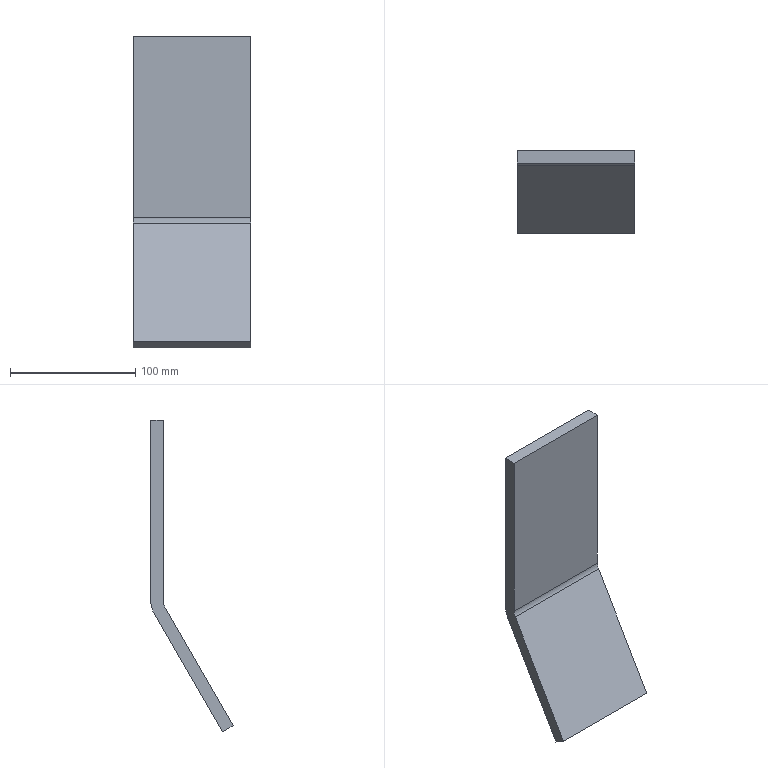Part | STEP file | VD-SYL0380DJ1006_1_4-5_VD-SYL03 | 1 solid | 10 faces | box 94 x 65.818 x 249 mm | volume 245764 mm3 | plane 8 | cylinder 2 | commonest cylinder face diameters 20 x1 40 x1
STEP:
#1=CARTESIAN_POINT('',(-47.,0.,-144.641));
#2=VERTEX_POINT('',#1);
#3=CARTESIAN_POINT('',(47.,0.,-144.641));
#4=VERTEX_POINT('',#3);
#5=CARTESIAN_POINT('',(-47.,0.,-144.641));
#6=DIRECTION('',(1.,0.,0.));
#7=VECTOR('',#6,1000.);
#8=LINE('',#5,#7);
#9=EDGE_CURVE('',#2,#4,#8,.T.);
#10=ORIENTED_EDGE('',*,*,#9,.F.);
#11=CARTESIAN_POINT('',(-47.,0.,0.));
#12=VERTEX_POINT('',#11);
#13=CARTESIAN_POINT('',(-47.,0.,0.));
#14=DIRECTION('',(0.,0.,-1.));
#15=VECTOR('',#14,1000.);
#16=LINE('',#13,#15);
#17=EDGE_CURVE('',#12,#2,#16,.T.);
#18=ORIENTED_EDGE('',*,*,#17,.F.);
#19=CARTESIAN_POINT('',(47.,0.,0.));
#20=VERTEX_POINT('',#19);
#21=CARTESIAN_POINT('',(47.,0.,0.));
#22=DIRECTION('',(-1.,0.,0.));
#23=VECTOR('',#22,1000.);
#24=LINE('',#21,#23);
#25=EDGE_CURVE('',#20,#12,#24,.T.);
#26=ORIENTED_EDGE('',*,*,#25,.F.);
#27=CARTESIAN_POINT('',(47.,0.,-144.641));
#28=DIRECTION('',(0.,0.,1.));
#29=VECTOR('',#28,1000.);
#30=LINE('',#27,#29);
#31=EDGE_CURVE('',#4,#20,#30,.T.);
#32=ORIENTED_EDGE('',*,*,#31,.F.);
#33=EDGE_LOOP('',(#10,#18,#26,#32));
#34=FACE_OUTER_BOUND('',#33,.T.);
#35=CARTESIAN_POINT('',(-47.,0.,-150.));
#36=DIRECTION('',(0.,1.,0.));
#37=DIRECTION('',(1.,0.,0.));
#38=AXIS2_PLACEMENT_3D('',#35,#36,#37);
#39=PLANE('',#38);
#40=ADVANCED_FACE('',(#34),#39,.T.);
#41=CARTESIAN_POINT('',(-47.,-2.679,-154.641));
#42=VERTEX_POINT('',#41);
#43=CARTESIAN_POINT('',(-47.,-20.,-144.641));
#44=DIRECTION('',(-1.,0.,0.));
#45=DIRECTION('',(0.,1.,0.));
#46=AXIS2_PLACEMENT_3D('',#43,#44,#45);
#47=CIRCLE('',#46,20.);
#48=EDGE_CURVE('',#2,#42,#47,.T.);
#49=ORIENTED_EDGE('',*,*,#48,.T.);
#50=CARTESIAN_POINT('',(-47.,-57.158,-249.));
#51=VERTEX_POINT('',#50);
#52=CARTESIAN_POINT('',(-47.,-2.679,-154.641));
#53=DIRECTION('',(0.,-0.5,-0.866));
#54=VECTOR('',#53,1000.);
#55=LINE('',#52,#54);
#56=EDGE_CURVE('',#42,#51,#55,.T.);
#57=ORIENTED_EDGE('',*,*,#56,.T.);
#58=CARTESIAN_POINT('',(-47.,-65.818,-244.));
#59=VERTEX_POINT('',#58);
#60=CARTESIAN_POINT('',(-47.,-57.158,-249.));
#61=DIRECTION('',(0.,-0.866,0.5));
#62=VECTOR('',#61,1000.);
#63=LINE('',#60,#62);
#64=EDGE_CURVE('',#51,#59,#63,.T.);
#65=ORIENTED_EDGE('',*,*,#64,.T.);
#66=CARTESIAN_POINT('',(-47.,-11.34,-149.641));
#67=VERTEX_POINT('',#66);
#68=CARTESIAN_POINT('',(-47.,-65.818,-244.));
#69=DIRECTION('',(0.,0.5,0.866));
#70=VECTOR('',#69,1000.);
#71=LINE('',#68,#70);
#72=EDGE_CURVE('',#59,#67,#71,.T.);
#73=ORIENTED_EDGE('',*,*,#72,.T.);
#74=CARTESIAN_POINT('',(-47.,-10.,-144.641));
#75=VERTEX_POINT('',#74);
#76=CARTESIAN_POINT('',(-47.,-20.,-144.641));
#77=DIRECTION('',(1.,0.,0.));
#78=DIRECTION('',(0.,0.866,-0.5));
#79=AXIS2_PLACEMENT_3D('',#76,#77,#78);
#80=CIRCLE('',#79,10.);
#81=EDGE_CURVE('',#67,#75,#80,.T.);
#82=ORIENTED_EDGE('',*,*,#81,.T.);
#83=CARTESIAN_POINT('',(-47.,-10.,0.));
#84=VERTEX_POINT('',#83);
#85=CARTESIAN_POINT('',(-47.,-10.,0.));
#86=DIRECTION('',(0.,0.,-1.));
#87=VECTOR('',#86,1000.);
#88=LINE('',#85,#87);
#89=EDGE_CURVE('',#84,#75,#88,.T.);
#90=ORIENTED_EDGE('',*,*,#89,.F.);
#91=CARTESIAN_POINT('',(-47.,-10.,0.));
#92=DIRECTION('',(0.,1.,0.));
#93=VECTOR('',#92,1000.);
#94=LINE('',#91,#93);
#95=EDGE_CURVE('',#84,#12,#94,.T.);
#96=ORIENTED_EDGE('',*,*,#95,.T.);
#97=ORIENTED_EDGE('',*,*,#17,.T.);
#98=EDGE_LOOP('',(#49,#57,#65,#73,#82,#90,#96,#97));
#99=FACE_OUTER_BOUND('',#98,.T.);
#100=CARTESIAN_POINT('',(-47.,-5.,-74.33));
#101=DIRECTION('',(-1.,0.,0.));
#102=DIRECTION('',(0.,0.,1.));
#103=AXIS2_PLACEMENT_3D('',#100,#101,#102);
#104=PLANE('',#103);
#105=ADVANCED_FACE('',(#99),#104,.T.);
#106=CARTESIAN_POINT('',(47.,-2.679,-154.641));
#107=VERTEX_POINT('',#106);
#108=CARTESIAN_POINT('',(47.,-2.679,-154.641));
#109=DIRECTION('',(-1.,0.,0.));
#110=VECTOR('',#109,1000.);
#111=LINE('',#108,#110);
#112=EDGE_CURVE('',#107,#42,#111,.T.);
#113=ORIENTED_EDGE('',*,*,#112,.F.);
#114=CARTESIAN_POINT('',(47.,-57.158,-249.));
#115=VERTEX_POINT('',#114);
#116=CARTESIAN_POINT('',(47.,-57.158,-249.));
#117=DIRECTION('',(0.,0.5,0.866));
#118=VECTOR('',#117,1000.);
#119=LINE('',#116,#118);
#120=EDGE_CURVE('',#115,#107,#119,.T.);
#121=ORIENTED_EDGE('',*,*,#120,.F.);
#122=CARTESIAN_POINT('',(-47.,-57.158,-249.));
#123=DIRECTION('',(1.,0.,0.));
#124=VECTOR('',#123,1000.);
#125=LINE('',#122,#124);
#126=EDGE_CURVE('',#51,#115,#125,.T.);
#127=ORIENTED_EDGE('',*,*,#126,.F.);
#128=ORIENTED_EDGE('',*,*,#56,.F.);
#129=EDGE_LOOP('',(#113,#121,#127,#128));
#130=FACE_OUTER_BOUND('',#129,.T.);
#131=CARTESIAN_POINT('',(-47.,-57.158,-249.));
#132=DIRECTION('',(0.,0.866,-0.5));
#133=DIRECTION('',(-1.,0.,0.));
#134=AXIS2_PLACEMENT_3D('',#131,#132,#133);
#135=PLANE('',#134);
#136=ADVANCED_FACE('',(#130),#135,.T.);
#137=ORIENTED_EDGE('',*,*,#64,.F.);
#138=ORIENTED_EDGE('',*,*,#126,.T.);
#139=CARTESIAN_POINT('',(47.,-65.818,-244.));
#140=VERTEX_POINT('',#139);
#141=CARTESIAN_POINT('',(47.,-65.818,-244.));
#142=DIRECTION('',(0.,0.866,-0.5));
#143=VECTOR('',#142,1000.);
#144=LINE('',#141,#143);
#145=EDGE_CURVE('',#140,#115,#144,.T.);
#146=ORIENTED_EDGE('',*,*,#145,.F.);
#147=CARTESIAN_POINT('',(47.,-65.818,-244.));
#148=DIRECTION('',(-1.,0.,0.));
#149=VECTOR('',#148,1000.);
#150=LINE('',#147,#149);
#151=EDGE_CURVE('',#140,#59,#150,.T.);
#152=ORIENTED_EDGE('',*,*,#151,.T.);
#153=EDGE_LOOP('',(#137,#138,#146,#152));
#154=FACE_OUTER_BOUND('',#153,.T.);
#155=CARTESIAN_POINT('',(0.,-61.488,-246.5));
#156=DIRECTION('',(0.,0.5,0.866));
#157=DIRECTION('',(1.,0.,0.));
#158=AXIS2_PLACEMENT_3D('',#155,#156,#157);
#159=PLANE('',#158);
#160=ADVANCED_FACE('',(#154),#159,.F.);
#161=CARTESIAN_POINT('',(47.,-11.34,-149.641));
#162=VERTEX_POINT('',#161);
#163=CARTESIAN_POINT('',(47.,-11.34,-149.641));
#164=DIRECTION('',(0.,-0.5,-0.866));
#165=VECTOR('',#164,1000.);
#166=LINE('',#163,#165);
#167=EDGE_CURVE('',#162,#140,#166,.T.);
#168=ORIENTED_EDGE('',*,*,#167,.F.);
#169=CARTESIAN_POINT('',(-47.,-11.34,-149.641));
#170=DIRECTION('',(1.,0.,0.));
#171=VECTOR('',#170,1000.);
#172=LINE('',#169,#171);
#173=EDGE_CURVE('',#67,#162,#172,.T.);
#174=ORIENTED_EDGE('',*,*,#173,.F.);
#175=ORIENTED_EDGE('',*,*,#72,.F.);
#176=ORIENTED_EDGE('',*,*,#151,.F.);
#177=EDGE_LOOP('',(#168,#174,#175,#176));
#178=FACE_OUTER_BOUND('',#177,.T.);
#179=CARTESIAN_POINT('',(-47.,-65.818,-244.));
#180=DIRECTION('',(0.,0.866,-0.5));
#181=DIRECTION('',(-1.,0.,0.));
#182=AXIS2_PLACEMENT_3D('',#179,#180,#181);
#183=PLANE('',#182);
#184=ADVANCED_FACE('',(#178),#183,.F.);
#185=ORIENTED_EDGE('',*,*,#81,.F.);
#186=ORIENTED_EDGE('',*,*,#173,.T.);
#187=CARTESIAN_POINT('',(47.,-10.,-144.641));
#188=VERTEX_POINT('',#187);
#189=CARTESIAN_POINT('',(47.,-20.,-144.641));
#190=DIRECTION('',(-1.,0.,0.));
#191=DIRECTION('',(0.,1.,0.));
#192=AXIS2_PLACEMENT_3D('',#189,#190,#191);
#193=CIRCLE('',#192,10.);
#194=EDGE_CURVE('',#188,#162,#193,.T.);
#195=ORIENTED_EDGE('',*,*,#194,.F.);
#196=CARTESIAN_POINT('',(47.,-10.,-144.641));
#197=DIRECTION('',(-1.,0.,0.));
#198=VECTOR('',#197,1000.);
#199=LINE('',#196,#198);
#200=EDGE_CURVE('',#188,#75,#199,.T.);
#201=ORIENTED_EDGE('',*,*,#200,.T.);
#202=EDGE_LOOP('',(#185,#186,#195,#201));
#203=FACE_OUTER_BOUND('',#202,.T.);
#204=CARTESIAN_POINT('',(266.029,-20.,-144.641));
#205=DIRECTION('',(-1.,0.,0.));
#206=DIRECTION('',(0.,0.,1.));
#207=AXIS2_PLACEMENT_3D('',#204,#205,#206);
#208=CYLINDRICAL_SURFACE('',#207,10.);
#209=ADVANCED_FACE('',(#203),#208,.F.);
#210=ORIENTED_EDGE('',*,*,#89,.T.);
#211=ORIENTED_EDGE('',*,*,#200,.F.);
#212=CARTESIAN_POINT('',(47.,-10.,0.));
#213=VERTEX_POINT('',#212);
#214=CARTESIAN_POINT('',(47.,-10.,0.));
#215=DIRECTION('',(0.,0.,-1.));
#216=VECTOR('',#215,1000.);
#217=LINE('',#214,#216);
#218=EDGE_CURVE('',#213,#188,#217,.T.);
#219=ORIENTED_EDGE('',*,*,#218,.F.);
#220=CARTESIAN_POINT('',(47.,-10.,0.));
#221=DIRECTION('',(-1.,0.,0.));
#222=VECTOR('',#221,1000.);
#223=LINE('',#220,#222);
#224=EDGE_CURVE('',#213,#84,#223,.T.);
#225=ORIENTED_EDGE('',*,*,#224,.T.);
#226=EDGE_LOOP('',(#210,#211,#219,#225));
#227=FACE_OUTER_BOUND('',#226,.T.);
#228=CARTESIAN_POINT('',(-47.,-10.,-150.));
#229=DIRECTION('',(0.,1.,0.));
#230=DIRECTION('',(1.,0.,0.));
#231=AXIS2_PLACEMENT_3D('',#228,#229,#230);
#232=PLANE('',#231);
#233=ADVANCED_FACE('',(#227),#232,.F.);
#234=ORIENTED_EDGE('',*,*,#25,.T.);
#235=ORIENTED_EDGE('',*,*,#95,.F.);
#236=ORIENTED_EDGE('',*,*,#224,.F.);
#237=CARTESIAN_POINT('',(47.,0.,0.));
#238=DIRECTION('',(0.,-1.,0.));
#239=VECTOR('',#238,1000.);
#240=LINE('',#237,#239);
#241=EDGE_CURVE('',#20,#213,#240,.T.);
#242=ORIENTED_EDGE('',*,*,#241,.F.);
#243=EDGE_LOOP('',(#234,#235,#236,#242));
#244=FACE_OUTER_BOUND('',#243,.T.);
#245=CARTESIAN_POINT('',(0.,-5.,0.));
#246=DIRECTION('',(0.,0.,1.));
#247=DIRECTION('',(1.,0.,0.));
#248=AXIS2_PLACEMENT_3D('',#245,#246,#247);
#249=PLANE('',#248);
#250=ADVANCED_FACE('',(#244),#249,.T.);
#251=ORIENTED_EDGE('',*,*,#218,.T.);
#252=ORIENTED_EDGE('',*,*,#194,.T.);
#253=ORIENTED_EDGE('',*,*,#167,.T.);
#254=ORIENTED_EDGE('',*,*,#145,.T.);
#255=ORIENTED_EDGE('',*,*,#120,.T.);
#256=CARTESIAN_POINT('',(47.,-20.,-144.641));
#257=DIRECTION('',(1.,0.,0.));
#258=DIRECTION('',(0.,0.866,-0.5));
#259=AXIS2_PLACEMENT_3D('',#256,#257,#258);
#260=CIRCLE('',#259,20.);
#261=EDGE_CURVE('',#107,#4,#260,.T.);
#262=ORIENTED_EDGE('',*,*,#261,.T.);
#263=ORIENTED_EDGE('',*,*,#31,.T.);
#264=ORIENTED_EDGE('',*,*,#241,.T.);
#265=EDGE_LOOP('',(#251,#252,#253,#254,#255,#262,#263,#264));
#266=FACE_OUTER_BOUND('',#265,.T.);
#267=CARTESIAN_POINT('',(47.,-5.,-74.33));
#268=DIRECTION('',(-1.,0.,0.));
#269=DIRECTION('',(0.,0.,1.));
#270=AXIS2_PLACEMENT_3D('',#267,#268,#269);
#271=PLANE('',#270);
#272=ADVANCED_FACE('',(#266),#271,.F.);
#273=ORIENTED_EDGE('',*,*,#112,.T.);
#274=ORIENTED_EDGE('',*,*,#48,.F.);
#275=ORIENTED_EDGE('',*,*,#9,.T.);
#276=ORIENTED_EDGE('',*,*,#261,.F.);
#277=EDGE_LOOP('',(#273,#274,#275,#276));
#278=FACE_OUTER_BOUND('',#277,.T.);
#279=CARTESIAN_POINT('',(266.029,-20.,-144.641));
#280=DIRECTION('',(-1.,0.,0.));
#281=DIRECTION('',(0.,0.,1.));
#282=AXIS2_PLACEMENT_3D('',#279,#280,#281);
#283=CYLINDRICAL_SURFACE('',#282,20.);
#284=ADVANCED_FACE('',(#278),#283,.T.);
#285=CLOSED_SHELL('',(#40,#105,#136,#160,#184,#209,#233,#250,#272,#284));
#286=MANIFOLD_SOLID_BREP('',#285);
#287=CARTESIAN_POINT('',(0.,0.,0.));
#288=DIRECTION('',(0.,0.,1.));
#289=DIRECTION('',(1.,0.,0.));
#290=AXIS2_PLACEMENT_3D('',#287,#288,#289);
#291=(LENGTH_UNIT()NAMED_UNIT(*)SI_UNIT(.MILLI.,.METRE.));
#292=UNCERTAINTY_MEASURE_WITH_UNIT(LENGTH_MEASURE(0.00001),#291,'','');
#293=(NAMED_UNIT(*)PLANE_ANGLE_UNIT()SI_UNIT($,.RADIAN.));
#294=(NAMED_UNIT(*)SI_UNIT($,.STERADIAN.)SOLID_ANGLE_UNIT());
#295=(GEOMETRIC_REPRESENTATION_CONTEXT(3)GLOBAL_UNCERTAINTY_ASSIGNED_CONTEXT((#292))GLOBAL_UNIT_ASSIGNED_CONTEXT((#291,#293,#294))REPRESENTATION_CONTEXT('',''));
#296=ADVANCED_BREP_SHAPE_REPRESENTATION('',(#286,#290),#295);